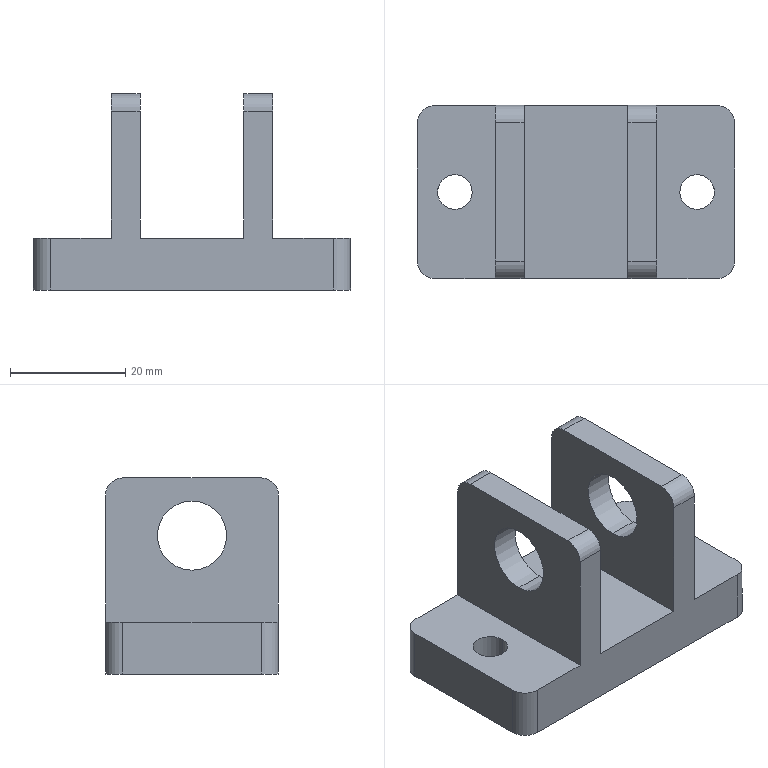Part | STEP file | Hinge seat | 1 solid | 30 faces | box 55 x 30 x 34 mm | volume 20602 mm3 | cylinder 16 | plane 14 | commonest cylinder face diameters 6 x12 12 x4
STEP:
#1=CARTESIAN_POINT('',(-24.,0.,0.));
#2=VERTEX_POINT('',#1);
#3=CARTESIAN_POINT('',(-18.,0.,0.));
#4=VERTEX_POINT('',#3);
#5=CARTESIAN_POINT('',(-21.,0.,0.));
#6=DIRECTION('',(0.,0.,1.));
#7=DIRECTION('',(1.,0.,0.));
#8=AXIS2_PLACEMENT_3D('',#5,#6,#7);
#9=CIRCLE('',#8,3.);
#10=EDGE_CURVE('',#2,#4,#9,.T.);
#11=ORIENTED_EDGE('',*,*,#10,.F.);
#12=CARTESIAN_POINT('',(-24.,0.,9.));
#13=VERTEX_POINT('',#12);
#14=CARTESIAN_POINT('',(-24.,0.,-11.));
#15=DIRECTION('',(0.,0.,1.));
#16=VECTOR('',#15,1000.);
#17=LINE('',#14,#16);
#18=EDGE_CURVE('',#2,#13,#17,.T.);
#19=ORIENTED_EDGE('',*,*,#18,.T.);
#20=CARTESIAN_POINT('',(-18.,0.,9.));
#21=VERTEX_POINT('',#20);
#22=CARTESIAN_POINT('',(-21.,0.,9.));
#23=DIRECTION('',(0.,0.,1.));
#24=DIRECTION('',(1.,0.,0.));
#25=AXIS2_PLACEMENT_3D('',#22,#23,#24);
#26=CIRCLE('',#25,3.);
#27=EDGE_CURVE('',#13,#21,#26,.T.);
#28=ORIENTED_EDGE('',*,*,#27,.T.);
#29=CARTESIAN_POINT('',(-18.,0.,-11.));
#30=DIRECTION('',(0.,0.,1.));
#31=VECTOR('',#30,1000.);
#32=LINE('',#29,#31);
#33=EDGE_CURVE('',#4,#21,#32,.T.);
#34=ORIENTED_EDGE('',*,*,#33,.F.);
#35=EDGE_LOOP('',(#11,#19,#28,#34));
#36=FACE_OUTER_BOUND('',#35,.T.);
#37=CARTESIAN_POINT('',(-21.,0.,-11.));
#38=DIRECTION('',(0.,0.,1.));
#39=DIRECTION('',(1.,0.,0.));
#40=AXIS2_PLACEMENT_3D('',#37,#38,#39);
#41=CYLINDRICAL_SURFACE('',#40,3.);
#42=ADVANCED_FACE('',(#36),#41,.F.);
#43=CARTESIAN_POINT('',(18.,0.,0.));
#44=VERTEX_POINT('',#43);
#45=CARTESIAN_POINT('',(24.,0.,0.));
#46=VERTEX_POINT('',#45);
#47=CARTESIAN_POINT('',(21.,0.,0.));
#48=DIRECTION('',(0.,0.,1.));
#49=DIRECTION('',(1.,0.,0.));
#50=AXIS2_PLACEMENT_3D('',#47,#48,#49);
#51=CIRCLE('',#50,3.);
#52=EDGE_CURVE('',#44,#46,#51,.T.);
#53=ORIENTED_EDGE('',*,*,#52,.F.);
#54=CARTESIAN_POINT('',(18.,0.,9.));
#55=VERTEX_POINT('',#54);
#56=CARTESIAN_POINT('',(18.,0.,-11.));
#57=DIRECTION('',(0.,0.,1.));
#58=VECTOR('',#57,1000.);
#59=LINE('',#56,#58);
#60=EDGE_CURVE('',#44,#55,#59,.T.);
#61=ORIENTED_EDGE('',*,*,#60,.T.);
#62=CARTESIAN_POINT('',(24.,0.,9.));
#63=VERTEX_POINT('',#62);
#64=CARTESIAN_POINT('',(21.,0.,9.));
#65=DIRECTION('',(0.,0.,1.));
#66=DIRECTION('',(1.,0.,0.));
#67=AXIS2_PLACEMENT_3D('',#64,#65,#66);
#68=CIRCLE('',#67,3.);
#69=EDGE_CURVE('',#55,#63,#68,.T.);
#70=ORIENTED_EDGE('',*,*,#69,.T.);
#71=CARTESIAN_POINT('',(24.,0.,-11.));
#72=DIRECTION('',(0.,0.,1.));
#73=VECTOR('',#72,1000.);
#74=LINE('',#71,#73);
#75=EDGE_CURVE('',#46,#63,#74,.T.);
#76=ORIENTED_EDGE('',*,*,#75,.F.);
#77=EDGE_LOOP('',(#53,#61,#70,#76));
#78=FACE_OUTER_BOUND('',#77,.T.);
#79=CARTESIAN_POINT('',(21.,0.,-11.));
#80=DIRECTION('',(0.,0.,1.));
#81=DIRECTION('',(1.,0.,0.));
#82=AXIS2_PLACEMENT_3D('',#79,#80,#81);
#83=CYLINDRICAL_SURFACE('',#82,3.);
#84=ADVANCED_FACE('',(#78),#83,.F.);
#85=CARTESIAN_POINT('',(-9.,0.,18.));
#86=VERTEX_POINT('',#85);
#87=CARTESIAN_POINT('',(-9.,0.,30.));
#88=VERTEX_POINT('',#87);
#89=CARTESIAN_POINT('',(-9.,0.,24.));
#90=DIRECTION('',(-1.,0.,0.));
#91=DIRECTION('',(0.,-1.,0.));
#92=AXIS2_PLACEMENT_3D('',#89,#90,#91);
#93=CIRCLE('',#92,6.);
#94=EDGE_CURVE('',#86,#88,#93,.T.);
#95=ORIENTED_EDGE('',*,*,#94,.F.);
#96=CARTESIAN_POINT('',(-14.,0.,18.));
#97=VERTEX_POINT('',#96);
#98=CARTESIAN_POINT('',(27.5,0.,18.));
#99=DIRECTION('',(-1.,0.,0.));
#100=VECTOR('',#99,1000.);
#101=LINE('',#98,#100);
#102=EDGE_CURVE('',#86,#97,#101,.T.);
#103=ORIENTED_EDGE('',*,*,#102,.T.);
#104=CARTESIAN_POINT('',(-14.,0.,30.));
#105=VERTEX_POINT('',#104);
#106=CARTESIAN_POINT('',(-14.,0.,24.));
#107=DIRECTION('',(-1.,0.,0.));
#108=DIRECTION('',(0.,0.,1.));
#109=AXIS2_PLACEMENT_3D('',#106,#107,#108);
#110=CIRCLE('',#109,6.);
#111=EDGE_CURVE('',#97,#105,#110,.T.);
#112=ORIENTED_EDGE('',*,*,#111,.T.);
#113=CARTESIAN_POINT('',(27.5,0.,30.));
#114=DIRECTION('',(-1.,0.,0.));
#115=VECTOR('',#114,1000.);
#116=LINE('',#113,#115);
#117=EDGE_CURVE('',#88,#105,#116,.T.);
#118=ORIENTED_EDGE('',*,*,#117,.F.);
#119=EDGE_LOOP('',(#95,#103,#112,#118));
#120=FACE_OUTER_BOUND('',#119,.T.);
#121=CARTESIAN_POINT('',(27.5,0.,24.));
#122=DIRECTION('',(-1.,0.,0.));
#123=DIRECTION('',(0.,0.,1.));
#124=AXIS2_PLACEMENT_3D('',#121,#122,#123);
#125=CYLINDRICAL_SURFACE('',#124,6.);
#126=ADVANCED_FACE('',(#120),#125,.F.);
#127=CARTESIAN_POINT('',(14.,0.,18.));
#128=VERTEX_POINT('',#127);
#129=CARTESIAN_POINT('',(14.,0.,30.));
#130=VERTEX_POINT('',#129);
#131=CARTESIAN_POINT('',(14.,0.,24.));
#132=DIRECTION('',(-1.,0.,0.));
#133=DIRECTION('',(0.,-1.,0.));
#134=AXIS2_PLACEMENT_3D('',#131,#132,#133);
#135=CIRCLE('',#134,6.);
#136=EDGE_CURVE('',#128,#130,#135,.T.);
#137=ORIENTED_EDGE('',*,*,#136,.F.);
#138=CARTESIAN_POINT('',(9.,0.,18.));
#139=VERTEX_POINT('',#138);
#140=CARTESIAN_POINT('',(27.5,0.,18.));
#141=DIRECTION('',(-1.,0.,0.));
#142=VECTOR('',#141,1000.);
#143=LINE('',#140,#142);
#144=EDGE_CURVE('',#128,#139,#143,.T.);
#145=ORIENTED_EDGE('',*,*,#144,.T.);
#146=CARTESIAN_POINT('',(9.,0.,30.));
#147=VERTEX_POINT('',#146);
#148=CARTESIAN_POINT('',(9.,0.,24.));
#149=DIRECTION('',(1.,0.,0.));
#150=DIRECTION('',(0.,1.,0.));
#151=AXIS2_PLACEMENT_3D('',#148,#149,#150);
#152=CIRCLE('',#151,6.);
#153=EDGE_CURVE('',#147,#139,#152,.T.);
#154=ORIENTED_EDGE('',*,*,#153,.F.);
#155=CARTESIAN_POINT('',(27.5,0.,30.));
#156=DIRECTION('',(-1.,0.,0.));
#157=VECTOR('',#156,1000.);
#158=LINE('',#155,#157);
#159=EDGE_CURVE('',#130,#147,#158,.T.);
#160=ORIENTED_EDGE('',*,*,#159,.F.);
#161=EDGE_LOOP('',(#137,#145,#154,#160));
#162=FACE_OUTER_BOUND('',#161,.T.);
#163=CARTESIAN_POINT('',(27.5,0.,24.));
#164=DIRECTION('',(-1.,0.,0.));
#165=DIRECTION('',(0.,0.,1.));
#166=AXIS2_PLACEMENT_3D('',#163,#164,#165);
#167=CYLINDRICAL_SURFACE('',#166,6.);
#168=ADVANCED_FACE('',(#162),#167,.F.);
#169=CARTESIAN_POINT('',(-9.,-15.,9.));
#170=VERTEX_POINT('',#169);
#171=CARTESIAN_POINT('',(9.,-15.,9.));
#172=VERTEX_POINT('',#171);
#173=CARTESIAN_POINT('',(-27.5,-15.,9.));
#174=DIRECTION('',(1.,0.,0.));
#175=VECTOR('',#174,1000.);
#176=LINE('',#173,#175);
#177=EDGE_CURVE('',#170,#172,#176,.T.);
#178=ORIENTED_EDGE('',*,*,#177,.T.);
#179=CARTESIAN_POINT('',(9.,15.,9.));
#180=VERTEX_POINT('',#179);
#181=CARTESIAN_POINT('',(9.,15.,9.));
#182=DIRECTION('',(0.,-1.,0.));
#183=VECTOR('',#182,1000.);
#184=LINE('',#181,#183);
#185=EDGE_CURVE('',#180,#172,#184,.T.);
#186=ORIENTED_EDGE('',*,*,#185,.F.);
#187=CARTESIAN_POINT('',(-9.,15.,9.));
#188=VERTEX_POINT('',#187);
#189=CARTESIAN_POINT('',(-27.5,15.,9.));
#190=DIRECTION('',(-1.,0.,0.));
#191=VECTOR('',#190,1000.);
#192=LINE('',#189,#191);
#193=EDGE_CURVE('',#180,#188,#192,.T.);
#194=ORIENTED_EDGE('',*,*,#193,.T.);
#195=CARTESIAN_POINT('',(-9.,15.,9.));
#196=DIRECTION('',(0.,1.,0.));
#197=VECTOR('',#196,1000.);
#198=LINE('',#195,#197);
#199=EDGE_CURVE('',#170,#188,#198,.T.);
#200=ORIENTED_EDGE('',*,*,#199,.F.);
#201=EDGE_LOOP('',(#178,#186,#194,#200));
#202=FACE_OUTER_BOUND('',#201,.T.);
#203=CARTESIAN_POINT('',(0.,0.,9.));
#204=DIRECTION('',(0.,0.,1.));
#205=DIRECTION('',(1.,0.,0.));
#206=AXIS2_PLACEMENT_3D('',#203,#204,#205);
#207=PLANE('',#206);
#208=ADVANCED_FACE('',(#202),#207,.T.);
#209=CARTESIAN_POINT('',(21.,0.,9.));
#210=DIRECTION('',(0.,0.,1.));
#211=DIRECTION('',(1.,0.,0.));
#212=AXIS2_PLACEMENT_3D('',#209,#210,#211);
#213=CIRCLE('',#212,3.);
#214=EDGE_CURVE('',#63,#55,#213,.T.);
#215=ORIENTED_EDGE('',*,*,#214,.F.);
#216=ORIENTED_EDGE('',*,*,#69,.F.);
#217=EDGE_LOOP('',(#215,#216));
#218=FACE_BOUND('',#217,.T.);
#219=CARTESIAN_POINT('',(24.5,15.,9.));
#220=VERTEX_POINT('',#219);
#221=CARTESIAN_POINT('',(14.,15.,9.));
#222=VERTEX_POINT('',#221);
#223=CARTESIAN_POINT('',(-27.5,15.,9.));
#224=DIRECTION('',(-1.,0.,0.));
#225=VECTOR('',#224,1000.);
#226=LINE('',#223,#225);
#227=EDGE_CURVE('',#220,#222,#226,.T.);
#228=ORIENTED_EDGE('',*,*,#227,.T.);
#229=CARTESIAN_POINT('',(14.,-15.,9.));
#230=VERTEX_POINT('',#229);
#231=CARTESIAN_POINT('',(14.,15.,9.));
#232=DIRECTION('',(0.,1.,0.));
#233=VECTOR('',#232,1000.);
#234=LINE('',#231,#233);
#235=EDGE_CURVE('',#230,#222,#234,.T.);
#236=ORIENTED_EDGE('',*,*,#235,.F.);
#237=CARTESIAN_POINT('',(24.5,-15.,9.));
#238=VERTEX_POINT('',#237);
#239=CARTESIAN_POINT('',(-27.5,-15.,9.));
#240=DIRECTION('',(1.,0.,0.));
#241=VECTOR('',#240,1000.);
#242=LINE('',#239,#241);
#243=EDGE_CURVE('',#230,#238,#242,.T.);
#244=ORIENTED_EDGE('',*,*,#243,.T.);
#245=CARTESIAN_POINT('',(27.5,-12.,9.));
#246=VERTEX_POINT('',#245);
#247=CARTESIAN_POINT('',(24.5,-12.,9.));
#248=DIRECTION('',(0.,0.,1.));
#249=DIRECTION('',(1.,0.,0.));
#250=AXIS2_PLACEMENT_3D('',#247,#248,#249);
#251=CIRCLE('',#250,3.);
#252=EDGE_CURVE('',#238,#246,#251,.T.);
#253=ORIENTED_EDGE('',*,*,#252,.T.);
#254=CARTESIAN_POINT('',(27.5,12.,9.));
#255=VERTEX_POINT('',#254);
#256=CARTESIAN_POINT('',(27.5,15.,9.));
#257=DIRECTION('',(0.,1.,0.));
#258=VECTOR('',#257,1000.);
#259=LINE('',#256,#258);
#260=EDGE_CURVE('',#246,#255,#259,.T.);
#261=ORIENTED_EDGE('',*,*,#260,.T.);
#262=CARTESIAN_POINT('',(24.5,12.,9.));
#263=DIRECTION('',(0.,0.,1.));
#264=DIRECTION('',(1.,0.,0.));
#265=AXIS2_PLACEMENT_3D('',#262,#263,#264);
#266=CIRCLE('',#265,3.);
#267=EDGE_CURVE('',#255,#220,#266,.T.);
#268=ORIENTED_EDGE('',*,*,#267,.T.);
#269=EDGE_LOOP('',(#228,#236,#244,#253,#261,#268));
#270=FACE_OUTER_BOUND('',#269,.T.);
#271=CARTESIAN_POINT('',(0.,0.,9.));
#272=DIRECTION('',(0.,0.,1.));
#273=DIRECTION('',(1.,0.,0.));
#274=AXIS2_PLACEMENT_3D('',#271,#272,#273);
#275=PLANE('',#274);
#276=ADVANCED_FACE('',(#218,#270),#275,.T.);
#277=CARTESIAN_POINT('',(-21.,0.,9.));
#278=DIRECTION('',(0.,0.,1.));
#279=DIRECTION('',(1.,0.,0.));
#280=AXIS2_PLACEMENT_3D('',#277,#278,#279);
#281=CIRCLE('',#280,3.);
#282=EDGE_CURVE('',#21,#13,#281,.T.);
#283=ORIENTED_EDGE('',*,*,#282,.F.);
#284=ORIENTED_EDGE('',*,*,#27,.F.);
#285=EDGE_LOOP('',(#283,#284));
#286=FACE_BOUND('',#285,.T.);
#287=CARTESIAN_POINT('',(-14.,15.,9.));
#288=VERTEX_POINT('',#287);
#289=CARTESIAN_POINT('',(-14.,-15.,9.));
#290=VERTEX_POINT('',#289);
#291=CARTESIAN_POINT('',(-14.,15.,9.));
#292=DIRECTION('',(0.,-1.,0.));
#293=VECTOR('',#292,1000.);
#294=LINE('',#291,#293);
#295=EDGE_CURVE('',#288,#290,#294,.T.);
#296=ORIENTED_EDGE('',*,*,#295,.F.);
#297=CARTESIAN_POINT('',(-24.5,15.,9.));
#298=VERTEX_POINT('',#297);
#299=CARTESIAN_POINT('',(-27.5,15.,9.));
#300=DIRECTION('',(-1.,0.,0.));
#301=VECTOR('',#300,1000.);
#302=LINE('',#299,#301);
#303=EDGE_CURVE('',#288,#298,#302,.T.);
#304=ORIENTED_EDGE('',*,*,#303,.T.);
#305=CARTESIAN_POINT('',(-27.5,12.,9.));
#306=VERTEX_POINT('',#305);
#307=CARTESIAN_POINT('',(-24.5,12.,9.));
#308=DIRECTION('',(0.,0.,1.));
#309=DIRECTION('',(1.,0.,0.));
#310=AXIS2_PLACEMENT_3D('',#307,#308,#309);
#311=CIRCLE('',#310,3.);
#312=EDGE_CURVE('',#298,#306,#311,.T.);
#313=ORIENTED_EDGE('',*,*,#312,.T.);
#314=CARTESIAN_POINT('',(-27.5,-12.,9.));
#315=VERTEX_POINT('',#314);
#316=CARTESIAN_POINT('',(-27.5,15.,9.));
#317=DIRECTION('',(0.,-1.,0.));
#318=VECTOR('',#317,1000.);
#319=LINE('',#316,#318);
#320=EDGE_CURVE('',#306,#315,#319,.T.);
#321=ORIENTED_EDGE('',*,*,#320,.T.);
#322=CARTESIAN_POINT('',(-24.5,-15.,9.));
#323=VERTEX_POINT('',#322);
#324=CARTESIAN_POINT('',(-24.5,-12.,9.));
#325=DIRECTION('',(0.,0.,1.));
#326=DIRECTION('',(1.,0.,0.));
#327=AXIS2_PLACEMENT_3D('',#324,#325,#326);
#328=CIRCLE('',#327,3.);
#329=EDGE_CURVE('',#315,#323,#328,.T.);
#330=ORIENTED_EDGE('',*,*,#329,.T.);
#331=CARTESIAN_POINT('',(-27.5,-15.,9.));
#332=DIRECTION('',(1.,0.,0.));
#333=VECTOR('',#332,1000.);
#334=LINE('',#331,#333);
#335=EDGE_CURVE('',#323,#290,#334,.T.);
#336=ORIENTED_EDGE('',*,*,#335,.T.);
#337=EDGE_LOOP('',(#296,#304,#313,#321,#330,#336));
#338=FACE_OUTER_BOUND('',#337,.T.);
#339=CARTESIAN_POINT('',(0.,0.,9.));
#340=DIRECTION('',(0.,0.,1.));
#341=DIRECTION('',(1.,0.,0.));
#342=AXIS2_PLACEMENT_3D('',#339,#340,#341);
#343=PLANE('',#342);
#344=ADVANCED_FACE('',(#286,#338),#343,.T.);
#345=CARTESIAN_POINT('',(27.5,-12.,0.));
#346=VERTEX_POINT('',#345);
#347=CARTESIAN_POINT('',(27.5,12.,0.));
#348=VERTEX_POINT('',#347);
#349=CARTESIAN_POINT('',(27.5,15.,0.));
#350=DIRECTION('',(0.,1.,0.));
#351=VECTOR('',#350,1000.);
#352=LINE('',#349,#351);
#353=EDGE_CURVE('',#346,#348,#352,.T.);
#354=ORIENTED_EDGE('',*,*,#353,.T.);
#355=CARTESIAN_POINT('',(27.5,12.,9.));
#356=DIRECTION('',(0.,0.,1.));
#357=VECTOR('',#356,1000.);
#358=LINE('',#355,#357);
#359=EDGE_CURVE('',#348,#255,#358,.T.);
#360=ORIENTED_EDGE('',*,*,#359,.T.);
#361=ORIENTED_EDGE('',*,*,#260,.F.);
#362=CARTESIAN_POINT('',(27.5,-12.,9.));
#363=DIRECTION('',(0.,0.,-1.));
#364=VECTOR('',#363,1000.);
#365=LINE('',#362,#364);
#366=EDGE_CURVE('',#246,#346,#365,.T.);
#367=ORIENTED_EDGE('',*,*,#366,.T.);
#368=EDGE_LOOP('',(#354,#360,#361,#367));
#369=FACE_OUTER_BOUND('',#368,.T.);
#370=CARTESIAN_POINT('',(27.5,15.,9.));
#371=DIRECTION('',(-1.,0.,0.));
#372=DIRECTION('',(0.,-1.,0.));
#373=AXIS2_PLACEMENT_3D('',#370,#371,#372);
#374=PLANE('',#373);
#375=ADVANCED_FACE('',(#369),#374,.F.);
#376=CARTESIAN_POINT('',(9.,15.,31.));
#377=VERTEX_POINT('',#376);
#378=CARTESIAN_POINT('',(9.,15.,34.));
#379=DIRECTION('',(0.,0.,-1.));
#380=VECTOR('',#379,1000.);
#381=LINE('',#378,#380);
#382=EDGE_CURVE('',#377,#180,#381,.T.);
#383=ORIENTED_EDGE('',*,*,#382,.F.);
#384=CARTESIAN_POINT('',(14.,15.,31.));
#385=VERTEX_POINT('',#384);
#386=CARTESIAN_POINT('',(14.,15.,31.));
#387=DIRECTION('',(1.,0.,0.));
#388=VECTOR('',#387,1000.);
#389=LINE('',#386,#388);
#390=EDGE_CURVE('',#377,#385,#389,.T.);
#391=ORIENTED_EDGE('',*,*,#390,.T.);
#392=CARTESIAN_POINT('',(14.,15.,34.));
#393=DIRECTION('',(0.,0.,-1.));
#394=VECTOR('',#393,1000.);
#395=LINE('',#392,#394);
#396=EDGE_CURVE('',#385,#222,#395,.T.);
#397=ORIENTED_EDGE('',*,*,#396,.T.);
#398=ORIENTED_EDGE('',*,*,#227,.F.);
#399=CARTESIAN_POINT('',(24.5,15.,0.));
#400=VERTEX_POINT('',#399);
#401=CARTESIAN_POINT('',(24.5,15.,9.));
#402=DIRECTION('',(0.,0.,-1.));
#403=VECTOR('',#402,1000.);
#404=LINE('',#401,#403);
#405=EDGE_CURVE('',#220,#400,#404,.T.);
#406=ORIENTED_EDGE('',*,*,#405,.T.);
#407=CARTESIAN_POINT('',(-24.5,15.,0.));
#408=VERTEX_POINT('',#407);
#409=CARTESIAN_POINT('',(-27.5,15.,0.));
#410=DIRECTION('',(-1.,0.,0.));
#411=VECTOR('',#410,1000.);
#412=LINE('',#409,#411);
#413=EDGE_CURVE('',#400,#408,#412,.T.);
#414=ORIENTED_EDGE('',*,*,#413,.T.);
#415=CARTESIAN_POINT('',(-24.5,15.,9.));
#416=DIRECTION('',(0.,0.,1.));
#417=VECTOR('',#416,1000.);
#418=LINE('',#415,#417);
#419=EDGE_CURVE('',#408,#298,#418,.T.);
#420=ORIENTED_EDGE('',*,*,#419,.T.);
#421=ORIENTED_EDGE('',*,*,#303,.F.);
#422=CARTESIAN_POINT('',(-14.,15.,31.));
#423=VERTEX_POINT('',#422);
#424=CARTESIAN_POINT('',(-14.,15.,34.));
#425=DIRECTION('',(0.,0.,-1.));
#426=VECTOR('',#425,1000.);
#427=LINE('',#424,#426);
#428=EDGE_CURVE('',#423,#288,#427,.T.);
#429=ORIENTED_EDGE('',*,*,#428,.F.);
#430=CARTESIAN_POINT('',(-9.,15.,31.));
#431=VERTEX_POINT('',#430);
#432=CARTESIAN_POINT('',(-9.,15.,31.));
#433=DIRECTION('',(1.,0.,0.));
#434=VECTOR('',#433,1000.);
#435=LINE('',#432,#434);
#436=EDGE_CURVE('',#423,#431,#435,.T.);
#437=ORIENTED_EDGE('',*,*,#436,.T.);
#438=CARTESIAN_POINT('',(-9.,15.,34.));
#439=DIRECTION('',(0.,0.,-1.));
#440=VECTOR('',#439,1000.);
#441=LINE('',#438,#440);
#442=EDGE_CURVE('',#431,#188,#441,.T.);
#443=ORIENTED_EDGE('',*,*,#442,.T.);
#444=ORIENTED_EDGE('',*,*,#193,.F.);
#445=EDGE_LOOP('',(#383,#391,#397,#398,#406,#414,#420,#421,#429,#437,#443,#444));
#446=FACE_OUTER_BOUND('',#445,.T.);
#447=CARTESIAN_POINT('',(-27.5,15.,9.));
#448=DIRECTION('',(0.,-1.,0.));
#449=DIRECTION('',(0.,0.,-1.));
#450=AXIS2_PLACEMENT_3D('',#447,#448,#449);
#451=PLANE('',#450);
#452=ADVANCED_FACE('',(#446),#451,.F.);
#453=ORIENTED_EDGE('',*,*,#320,.F.);
#454=CARTESIAN_POINT('',(-27.5,12.,0.));
#455=VERTEX_POINT('',#454);
#456=CARTESIAN_POINT('',(-27.5,12.,9.));
#457=DIRECTION('',(0.,0.,-1.));
#458=VECTOR('',#457,1000.);
#459=LINE('',#456,#458);
#460=EDGE_CURVE('',#306,#455,#459,.T.);
#461=ORIENTED_EDGE('',*,*,#460,.T.);
#462=CARTESIAN_POINT('',(-27.5,-12.,0.));
#463=VERTEX_POINT('',#462);
#464=CARTESIAN_POINT('',(-27.5,15.,0.));
#465=DIRECTION('',(0.,-1.,0.));
#466=VECTOR('',#465,1000.);
#467=LINE('',#464,#466);
#468=EDGE_CURVE('',#455,#463,#467,.T.);
#469=ORIENTED_EDGE('',*,*,#468,.T.);
#470=CARTESIAN_POINT('',(-27.5,-12.,9.));
#471=DIRECTION('',(0.,0.,1.));
#472=VECTOR('',#471,1000.);
#473=LINE('',#470,#472);
#474=EDGE_CURVE('',#463,#315,#473,.T.);
#475=ORIENTED_EDGE('',*,*,#474,.T.);
#476=EDGE_LOOP('',(#453,#461,#469,#475));
#477=FACE_OUTER_BOUND('',#476,.T.);
#478=CARTESIAN_POINT('',(-27.5,15.,9.));
#479=DIRECTION('',(1.,0.,0.));
#480=DIRECTION('',(0.,1.,0.));
#481=AXIS2_PLACEMENT_3D('',#478,#479,#480);
#482=PLANE('',#481);
#483=ADVANCED_FACE('',(#477),#482,.F.);
#484=CARTESIAN_POINT('',(14.,-15.,31.));
#485=VERTEX_POINT('',#484);
#486=CARTESIAN_POINT('',(14.,-15.,34.));
#487=DIRECTION('',(0.,0.,-1.));
#488=VECTOR('',#487,1000.);
#489=LINE('',#486,#488);
#490=EDGE_CURVE('',#485,#230,#489,.T.);
#491=ORIENTED_EDGE('',*,*,#490,.F.);
#492=CARTESIAN_POINT('',(9.,-15.,31.));
#493=VERTEX_POINT('',#492);
#494=CARTESIAN_POINT('',(9.,-15.,31.));
#495=DIRECTION('',(-1.,0.,0.));
#496=VECTOR('',#495,1000.);
#497=LINE('',#494,#496);
#498=EDGE_CURVE('',#485,#493,#497,.T.);
#499=ORIENTED_EDGE('',*,*,#498,.T.);
#500=CARTESIAN_POINT('',(9.,-15.,34.));
#501=DIRECTION('',(0.,0.,-1.));
#502=VECTOR('',#501,1000.);
#503=LINE('',#500,#502);
#504=EDGE_CURVE('',#493,#172,#503,.T.);
#505=ORIENTED_EDGE('',*,*,#504,.T.);
#506=ORIENTED_EDGE('',*,*,#177,.F.);
#507=CARTESIAN_POINT('',(-9.,-15.,31.));
#508=VERTEX_POINT('',#507);
#509=CARTESIAN_POINT('',(-9.,-15.,34.));
#510=DIRECTION('',(0.,0.,-1.));
#511=VECTOR('',#510,1000.);
#512=LINE('',#509,#511);
#513=EDGE_CURVE('',#508,#170,#512,.T.);
#514=ORIENTED_EDGE('',*,*,#513,.F.);
#515=CARTESIAN_POINT('',(-14.,-15.,31.));
#516=VERTEX_POINT('',#515);
#517=CARTESIAN_POINT('',(-14.,-15.,31.));
#518=DIRECTION('',(-1.,0.,0.));
#519=VECTOR('',#518,1000.);
#520=LINE('',#517,#519);
#521=EDGE_CURVE('',#508,#516,#520,.T.);
#522=ORIENTED_EDGE('',*,*,#521,.T.);
#523=CARTESIAN_POINT('',(-14.,-15.,34.));
#524=DIRECTION('',(0.,0.,-1.));
#525=VECTOR('',#524,1000.);
#526=LINE('',#523,#525);
#527=EDGE_CURVE('',#516,#290,#526,.T.);
#528=ORIENTED_EDGE('',*,*,#527,.T.);
#529=ORIENTED_EDGE('',*,*,#335,.F.);
#530=CARTESIAN_POINT('',(-24.5,-15.,0.));
#531=VERTEX_POINT('',#530);
#532=CARTESIAN_POINT('',(-24.5,-15.,9.));
#533=DIRECTION('',(0.,0.,-1.));
#534=VECTOR('',#533,1000.);
#535=LINE('',#532,#534);
#536=EDGE_CURVE('',#323,#531,#535,.T.);
#537=ORIENTED_EDGE('',*,*,#536,.T.);
#538=CARTESIAN_POINT('',(24.5,-15.,0.));
#539=VERTEX_POINT('',#538);
#540=CARTESIAN_POINT('',(-27.5,-15.,0.));
#541=DIRECTION('',(1.,0.,0.));
#542=VECTOR('',#541,1000.);
#543=LINE('',#540,#542);
#544=EDGE_CURVE('',#531,#539,#543,.T.);
#545=ORIENTED_EDGE('',*,*,#544,.T.);
#546=CARTESIAN_POINT('',(24.5,-15.,9.));
#547=DIRECTION('',(0.,0.,1.));
#548=VECTOR('',#547,1000.);
#549=LINE('',#546,#548);
#550=EDGE_CURVE('',#539,#238,#549,.T.);
#551=ORIENTED_EDGE('',*,*,#550,.T.);
#552=ORIENTED_EDGE('',*,*,#243,.F.);
#553=EDGE_LOOP('',(#491,#499,#505,#506,#514,#522,#528,#529,#537,#545,#551,#552));
#554=FACE_OUTER_BOUND('',#553,.T.);
#555=CARTESIAN_POINT('',(-27.5,-15.,9.));
#556=DIRECTION('',(0.,1.,0.));
#557=DIRECTION('',(0.,0.,1.));
#558=AXIS2_PLACEMENT_3D('',#555,#556,#557);
#559=PLANE('',#558);
#560=ADVANCED_FACE('',(#554),#559,.F.);
#561=CARTESIAN_POINT('',(-21.,0.,0.));
#562=DIRECTION('',(0.,0.,1.));
#563=DIRECTION('',(1.,0.,0.));
#564=AXIS2_PLACEMENT_3D('',#561,#562,#563);
#565=CIRCLE('',#564,3.);
#566=EDGE_CURVE('',#4,#2,#565,.T.);
#567=ORIENTED_EDGE('',*,*,#566,.T.);
#568=ORIENTED_EDGE('',*,*,#10,.T.);
#569=EDGE_LOOP('',(#567,#568));
#570=FACE_BOUND('',#569,.T.);
#571=CARTESIAN_POINT('',(21.,0.,0.));
#572=DIRECTION('',(0.,0.,1.));
#573=DIRECTION('',(1.,0.,0.));
#574=AXIS2_PLACEMENT_3D('',#571,#572,#573);
#575=CIRCLE('',#574,3.);
#576=EDGE_CURVE('',#46,#44,#575,.T.);
#577=ORIENTED_EDGE('',*,*,#576,.T.);
#578=ORIENTED_EDGE('',*,*,#52,.T.);
#579=EDGE_LOOP('',(#577,#578));
#580=FACE_BOUND('',#579,.T.);
#581=ORIENTED_EDGE('',*,*,#413,.F.);
#582=CARTESIAN_POINT('',(24.5,12.,0.));
#583=DIRECTION('',(0.,0.,-1.));
#584=DIRECTION('',(1.,0.,0.));
#585=AXIS2_PLACEMENT_3D('',#582,#583,#584);
#586=CIRCLE('',#585,3.);
#587=EDGE_CURVE('',#400,#348,#586,.T.);
#588=ORIENTED_EDGE('',*,*,#587,.T.);
#589=ORIENTED_EDGE('',*,*,#353,.F.);
#590=CARTESIAN_POINT('',(24.5,-12.,0.));
#591=DIRECTION('',(0.,0.,-1.));
#592=DIRECTION('',(1.,0.,0.));
#593=AXIS2_PLACEMENT_3D('',#590,#591,#592);
#594=CIRCLE('',#593,3.);
#595=EDGE_CURVE('',#346,#539,#594,.T.);
#596=ORIENTED_EDGE('',*,*,#595,.T.);
#597=ORIENTED_EDGE('',*,*,#544,.F.);
#598=CARTESIAN_POINT('',(-24.5,-12.,0.));
#599=DIRECTION('',(0.,0.,-1.));
#600=DIRECTION('',(1.,0.,0.));
#601=AXIS2_PLACEMENT_3D('',#598,#599,#600);
#602=CIRCLE('',#601,3.);
#603=EDGE_CURVE('',#531,#463,#602,.T.);
#604=ORIENTED_EDGE('',*,*,#603,.T.);
#605=ORIENTED_EDGE('',*,*,#468,.F.);
#606=CARTESIAN_POINT('',(-24.5,12.,0.));
#607=DIRECTION('',(0.,0.,-1.));
#608=DIRECTION('',(1.,0.,0.));
#609=AXIS2_PLACEMENT_3D('',#606,#607,#608);
#610=CIRCLE('',#609,3.);
#611=EDGE_CURVE('',#455,#408,#610,.T.);
#612=ORIENTED_EDGE('',*,*,#611,.T.);
#613=EDGE_LOOP('',(#581,#588,#589,#596,#597,#604,#605,#612));
#614=FACE_OUTER_BOUND('',#613,.T.);
#615=CARTESIAN_POINT('',(0.,0.,0.));
#616=DIRECTION('',(0.,0.,1.));
#617=DIRECTION('',(1.,0.,0.));
#618=AXIS2_PLACEMENT_3D('',#615,#616,#617);
#619=PLANE('',#618);
#620=ADVANCED_FACE('',(#570,#580,#614),#619,.F.);
#621=ORIENTED_EDGE('',*,*,#267,.F.);
#622=ORIENTED_EDGE('',*,*,#359,.F.);
#623=ORIENTED_EDGE('',*,*,#587,.F.);
#624=ORIENTED_EDGE('',*,*,#405,.F.);
#625=EDGE_LOOP('',(#621,#622,#623,#624));
#626=FACE_OUTER_BOUND('',#625,.T.);
#627=CARTESIAN_POINT('',(24.5,12.,9.));
#628=DIRECTION('',(0.,0.,-1.));
#629=DIRECTION('',(-1.,0.,0.));
#630=AXIS2_PLACEMENT_3D('',#627,#628,#629);
#631=CYLINDRICAL_SURFACE('',#630,3.);
#632=ADVANCED_FACE('',(#626),#631,.T.);
#633=ORIENTED_EDGE('',*,*,#252,.F.);
#634=ORIENTED_EDGE('',*,*,#550,.F.);
#635=ORIENTED_EDGE('',*,*,#595,.F.);
#636=ORIENTED_EDGE('',*,*,#366,.F.);
#637=EDGE_LOOP('',(#633,#634,#635,#636));
#638=FACE_OUTER_BOUND('',#637,.T.);
#639=CARTESIAN_POINT('',(24.5,-12.,9.));
#640=DIRECTION('',(0.,0.,-1.));
#641=DIRECTION('',(-1.,0.,0.));
#642=AXIS2_PLACEMENT_3D('',#639,#640,#641);
#643=CYLINDRICAL_SURFACE('',#642,3.);
#644=ADVANCED_FACE('',(#638),#643,.T.);
#645=ORIENTED_EDGE('',*,*,#312,.F.);
#646=ORIENTED_EDGE('',*,*,#419,.F.);
#647=ORIENTED_EDGE('',*,*,#611,.F.);
#648=ORIENTED_EDGE('',*,*,#460,.F.);
#649=EDGE_LOOP('',(#645,#646,#647,#648));
#650=FACE_OUTER_BOUND('',#649,.T.);
#651=CARTESIAN_POINT('',(-24.5,12.,9.));
#652=DIRECTION('',(0.,0.,-1.));
#653=DIRECTION('',(-1.,0.,0.));
#654=AXIS2_PLACEMENT_3D('',#651,#652,#653);
#655=CYLINDRICAL_SURFACE('',#654,3.);
#656=ADVANCED_FACE('',(#650),#655,.T.);
#657=ORIENTED_EDGE('',*,*,#329,.F.);
#658=ORIENTED_EDGE('',*,*,#474,.F.);
#659=ORIENTED_EDGE('',*,*,#603,.F.);
#660=ORIENTED_EDGE('',*,*,#536,.F.);
#661=EDGE_LOOP('',(#657,#658,#659,#660));
#662=FACE_OUTER_BOUND('',#661,.T.);
#663=CARTESIAN_POINT('',(-24.5,-12.,9.));
#664=DIRECTION('',(0.,0.,-1.));
#665=DIRECTION('',(-1.,0.,0.));
#666=AXIS2_PLACEMENT_3D('',#663,#664,#665);
#667=CYLINDRICAL_SURFACE('',#666,3.);
#668=ADVANCED_FACE('',(#662),#667,.T.);
#669=CARTESIAN_POINT('',(-14.,0.,24.));
#670=DIRECTION('',(-1.,0.,0.));
#671=DIRECTION('',(0.,0.,1.));
#672=AXIS2_PLACEMENT_3D('',#669,#670,#671);
#673=CIRCLE('',#672,6.);
#674=EDGE_CURVE('',#105,#97,#673,.T.);
#675=ORIENTED_EDGE('',*,*,#674,.F.);
#676=ORIENTED_EDGE('',*,*,#111,.F.);
#677=EDGE_LOOP('',(#675,#676));
#678=FACE_BOUND('',#677,.T.);
#679=ORIENTED_EDGE('',*,*,#527,.F.);
#680=CARTESIAN_POINT('',(-14.,-12.,34.));
#681=VERTEX_POINT('',#680);
#682=CARTESIAN_POINT('',(-14.,-12.,31.));
#683=DIRECTION('',(-1.,0.,0.));
#684=DIRECTION('',(0.,1.,0.));
#685=AXIS2_PLACEMENT_3D('',#682,#683,#684);
#686=CIRCLE('',#685,3.);
#687=EDGE_CURVE('',#516,#681,#686,.T.);
#688=ORIENTED_EDGE('',*,*,#687,.T.);
#689=CARTESIAN_POINT('',(-14.,12.,34.));
#690=VERTEX_POINT('',#689);
#691=CARTESIAN_POINT('',(-14.,15.,34.));
#692=DIRECTION('',(0.,-1.,0.));
#693=VECTOR('',#692,1000.);
#694=LINE('',#691,#693);
#695=EDGE_CURVE('',#690,#681,#694,.T.);
#696=ORIENTED_EDGE('',*,*,#695,.F.);
#697=CARTESIAN_POINT('',(-14.,12.,31.));
#698=DIRECTION('',(-1.,0.,0.));
#699=DIRECTION('',(0.,1.,0.));
#700=AXIS2_PLACEMENT_3D('',#697,#698,#699);
#701=CIRCLE('',#700,3.);
#702=EDGE_CURVE('',#690,#423,#701,.T.);
#703=ORIENTED_EDGE('',*,*,#702,.T.);
#704=ORIENTED_EDGE('',*,*,#428,.T.);
#705=ORIENTED_EDGE('',*,*,#295,.T.);
#706=EDGE_LOOP('',(#679,#688,#696,#703,#704,#705));
#707=FACE_OUTER_BOUND('',#706,.T.);
#708=CARTESIAN_POINT('',(-14.,15.,34.));
#709=DIRECTION('',(1.,0.,0.));
#710=DIRECTION('',(0.,1.,0.));
#711=AXIS2_PLACEMENT_3D('',#708,#709,#710);
#712=PLANE('',#711);
#713=ADVANCED_FACE('',(#678,#707),#712,.F.);
#714=CARTESIAN_POINT('',(-9.,0.,24.));
#715=DIRECTION('',(-1.,0.,0.));
#716=DIRECTION('',(0.,-1.,0.));
#717=AXIS2_PLACEMENT_3D('',#714,#715,#716);
#718=CIRCLE('',#717,6.);
#719=EDGE_CURVE('',#88,#86,#718,.T.);
#720=ORIENTED_EDGE('',*,*,#719,.T.);
#721=ORIENTED_EDGE('',*,*,#94,.T.);
#722=EDGE_LOOP('',(#720,#721));
#723=FACE_BOUND('',#722,.T.);
#724=CARTESIAN_POINT('',(-9.,-12.,34.));
#725=VERTEX_POINT('',#724);
#726=CARTESIAN_POINT('',(-9.,12.,34.));
#727=VERTEX_POINT('',#726);
#728=CARTESIAN_POINT('',(-9.,15.,34.));
#729=DIRECTION('',(0.,1.,0.));
#730=VECTOR('',#729,1000.);
#731=LINE('',#728,#730);
#732=EDGE_CURVE('',#725,#727,#731,.T.);
#733=ORIENTED_EDGE('',*,*,#732,.F.);
#734=CARTESIAN_POINT('',(-9.,-12.,31.));
#735=DIRECTION('',(1.,0.,0.));
#736=DIRECTION('',(0.,-1.,0.));
#737=AXIS2_PLACEMENT_3D('',#734,#735,#736);
#738=CIRCLE('',#737,3.);
#739=EDGE_CURVE('',#725,#508,#738,.T.);
#740=ORIENTED_EDGE('',*,*,#739,.T.);
#741=ORIENTED_EDGE('',*,*,#513,.T.);
#742=ORIENTED_EDGE('',*,*,#199,.T.);
#743=ORIENTED_EDGE('',*,*,#442,.F.);
#744=CARTESIAN_POINT('',(-9.,12.,31.));
#745=DIRECTION('',(1.,0.,0.));
#746=DIRECTION('',(0.,-1.,0.));
#747=AXIS2_PLACEMENT_3D('',#744,#745,#746);
#748=CIRCLE('',#747,3.);
#749=EDGE_CURVE('',#431,#727,#748,.T.);
#750=ORIENTED_EDGE('',*,*,#749,.T.);
#751=EDGE_LOOP('',(#733,#740,#741,#742,#743,#750));
#752=FACE_OUTER_BOUND('',#751,.T.);
#753=CARTESIAN_POINT('',(-9.,15.,34.));
#754=DIRECTION('',(-1.,0.,0.));
#755=DIRECTION('',(0.,-1.,0.));
#756=AXIS2_PLACEMENT_3D('',#753,#754,#755);
#757=PLANE('',#756);
#758=ADVANCED_FACE('',(#723,#752),#757,.F.);
#759=ORIENTED_EDGE('',*,*,#695,.T.);
#760=CARTESIAN_POINT('',(-9.,-12.,34.));
#761=DIRECTION('',(1.,0.,0.));
#762=VECTOR('',#761,1000.);
#763=LINE('',#760,#762);
#764=EDGE_CURVE('',#681,#725,#763,.T.);
#765=ORIENTED_EDGE('',*,*,#764,.T.);
#766=ORIENTED_EDGE('',*,*,#732,.T.);
#767=CARTESIAN_POINT('',(-14.,12.,34.));
#768=DIRECTION('',(-1.,0.,0.));
#769=VECTOR('',#768,1000.);
#770=LINE('',#767,#769);
#771=EDGE_CURVE('',#727,#690,#770,.T.);
#772=ORIENTED_EDGE('',*,*,#771,.T.);
#773=EDGE_LOOP('',(#759,#765,#766,#772));
#774=FACE_OUTER_BOUND('',#773,.T.);
#775=CARTESIAN_POINT('',(0.,0.,34.));
#776=DIRECTION('',(0.,0.,1.));
#777=DIRECTION('',(1.,0.,0.));
#778=AXIS2_PLACEMENT_3D('',#775,#776,#777);
#779=PLANE('',#778);
#780=ADVANCED_FACE('',(#774),#779,.T.);
#781=ORIENTED_EDGE('',*,*,#153,.T.);
#782=CARTESIAN_POINT('',(9.,0.,24.));
#783=DIRECTION('',(1.,0.,0.));
#784=DIRECTION('',(0.,1.,0.));
#785=AXIS2_PLACEMENT_3D('',#782,#783,#784);
#786=CIRCLE('',#785,6.);
#787=EDGE_CURVE('',#139,#147,#786,.T.);
#788=ORIENTED_EDGE('',*,*,#787,.T.);
#789=EDGE_LOOP('',(#781,#788));
#790=FACE_BOUND('',#789,.T.);
#791=ORIENTED_EDGE('',*,*,#504,.F.);
#792=CARTESIAN_POINT('',(9.,-12.,34.));
#793=VERTEX_POINT('',#792);
#794=CARTESIAN_POINT('',(9.,-12.,31.));
#795=DIRECTION('',(-1.,0.,0.));
#796=DIRECTION('',(0.,1.,0.));
#797=AXIS2_PLACEMENT_3D('',#794,#795,#796);
#798=CIRCLE('',#797,3.);
#799=EDGE_CURVE('',#493,#793,#798,.T.);
#800=ORIENTED_EDGE('',*,*,#799,.T.);
#801=CARTESIAN_POINT('',(9.,12.,34.));
#802=VERTEX_POINT('',#801);
#803=CARTESIAN_POINT('',(9.,15.,34.));
#804=DIRECTION('',(0.,-1.,0.));
#805=VECTOR('',#804,1000.);
#806=LINE('',#803,#805);
#807=EDGE_CURVE('',#802,#793,#806,.T.);
#808=ORIENTED_EDGE('',*,*,#807,.F.);
#809=CARTESIAN_POINT('',(9.,12.,31.));
#810=DIRECTION('',(-1.,0.,0.));
#811=DIRECTION('',(0.,1.,0.));
#812=AXIS2_PLACEMENT_3D('',#809,#810,#811);
#813=CIRCLE('',#812,3.);
#814=EDGE_CURVE('',#802,#377,#813,.T.);
#815=ORIENTED_EDGE('',*,*,#814,.T.);
#816=ORIENTED_EDGE('',*,*,#382,.T.);
#817=ORIENTED_EDGE('',*,*,#185,.T.);
#818=EDGE_LOOP('',(#791,#800,#808,#815,#816,#817));
#819=FACE_OUTER_BOUND('',#818,.T.);
#820=CARTESIAN_POINT('',(9.,15.,34.));
#821=DIRECTION('',(1.,0.,0.));
#822=DIRECTION('',(0.,1.,0.));
#823=AXIS2_PLACEMENT_3D('',#820,#821,#822);
#824=PLANE('',#823);
#825=ADVANCED_FACE('',(#790,#819),#824,.F.);
#826=CARTESIAN_POINT('',(14.,0.,24.));
#827=DIRECTION('',(-1.,0.,0.));
#828=DIRECTION('',(0.,-1.,0.));
#829=AXIS2_PLACEMENT_3D('',#826,#827,#828);
#830=CIRCLE('',#829,6.);
#831=EDGE_CURVE('',#130,#128,#830,.T.);
#832=ORIENTED_EDGE('',*,*,#831,.T.);
#833=ORIENTED_EDGE('',*,*,#136,.T.);
#834=EDGE_LOOP('',(#832,#833));
#835=FACE_BOUND('',#834,.T.);
#836=CARTESIAN_POINT('',(14.,-12.,34.));
#837=VERTEX_POINT('',#836);
#838=CARTESIAN_POINT('',(14.,12.,34.));
#839=VERTEX_POINT('',#838);
#840=CARTESIAN_POINT('',(14.,15.,34.));
#841=DIRECTION('',(0.,1.,0.));
#842=VECTOR('',#841,1000.);
#843=LINE('',#840,#842);
#844=EDGE_CURVE('',#837,#839,#843,.T.);
#845=ORIENTED_EDGE('',*,*,#844,.F.);
#846=CARTESIAN_POINT('',(14.,-12.,31.));
#847=DIRECTION('',(1.,0.,0.));
#848=DIRECTION('',(0.,-1.,0.));
#849=AXIS2_PLACEMENT_3D('',#846,#847,#848);
#850=CIRCLE('',#849,3.);
#851=EDGE_CURVE('',#837,#485,#850,.T.);
#852=ORIENTED_EDGE('',*,*,#851,.T.);
#853=ORIENTED_EDGE('',*,*,#490,.T.);
#854=ORIENTED_EDGE('',*,*,#235,.T.);
#855=ORIENTED_EDGE('',*,*,#396,.F.);
#856=CARTESIAN_POINT('',(14.,12.,31.));
#857=DIRECTION('',(1.,0.,0.));
#858=DIRECTION('',(0.,-1.,0.));
#859=AXIS2_PLACEMENT_3D('',#856,#857,#858);
#860=CIRCLE('',#859,3.);
#861=EDGE_CURVE('',#385,#839,#860,.T.);
#862=ORIENTED_EDGE('',*,*,#861,.T.);
#863=EDGE_LOOP('',(#845,#852,#853,#854,#855,#862));
#864=FACE_OUTER_BOUND('',#863,.T.);
#865=CARTESIAN_POINT('',(14.,15.,34.));
#866=DIRECTION('',(-1.,0.,0.));
#867=DIRECTION('',(0.,-1.,0.));
#868=AXIS2_PLACEMENT_3D('',#865,#866,#867);
#869=PLANE('',#868);
#870=ADVANCED_FACE('',(#835,#864),#869,.F.);
#871=ORIENTED_EDGE('',*,*,#807,.T.);
#872=CARTESIAN_POINT('',(14.,-12.,34.));
#873=DIRECTION('',(1.,0.,0.));
#874=VECTOR('',#873,1000.);
#875=LINE('',#872,#874);
#876=EDGE_CURVE('',#793,#837,#875,.T.);
#877=ORIENTED_EDGE('',*,*,#876,.T.);
#878=ORIENTED_EDGE('',*,*,#844,.T.);
#879=CARTESIAN_POINT('',(9.,12.,34.));
#880=DIRECTION('',(-1.,0.,0.));
#881=VECTOR('',#880,1000.);
#882=LINE('',#879,#881);
#883=EDGE_CURVE('',#839,#802,#882,.T.);
#884=ORIENTED_EDGE('',*,*,#883,.T.);
#885=EDGE_LOOP('',(#871,#877,#878,#884));
#886=FACE_OUTER_BOUND('',#885,.T.);
#887=CARTESIAN_POINT('',(0.,0.,34.));
#888=DIRECTION('',(0.,0.,1.));
#889=DIRECTION('',(1.,0.,0.));
#890=AXIS2_PLACEMENT_3D('',#887,#888,#889);
#891=PLANE('',#890);
#892=ADVANCED_FACE('',(#886),#891,.T.);
#893=ORIENTED_EDGE('',*,*,#799,.F.);
#894=ORIENTED_EDGE('',*,*,#498,.F.);
#895=ORIENTED_EDGE('',*,*,#851,.F.);
#896=ORIENTED_EDGE('',*,*,#876,.F.);
#897=EDGE_LOOP('',(#893,#894,#895,#896));
#898=FACE_OUTER_BOUND('',#897,.T.);
#899=CARTESIAN_POINT('',(0.,-12.,31.));
#900=DIRECTION('',(-1.,0.,0.));
#901=DIRECTION('',(0.,0.,1.));
#902=AXIS2_PLACEMENT_3D('',#899,#900,#901);
#903=CYLINDRICAL_SURFACE('',#902,3.);
#904=ADVANCED_FACE('',(#898),#903,.T.);
#905=ORIENTED_EDGE('',*,*,#687,.F.);
#906=ORIENTED_EDGE('',*,*,#521,.F.);
#907=ORIENTED_EDGE('',*,*,#739,.F.);
#908=ORIENTED_EDGE('',*,*,#764,.F.);
#909=EDGE_LOOP('',(#905,#906,#907,#908));
#910=FACE_OUTER_BOUND('',#909,.T.);
#911=CARTESIAN_POINT('',(0.,-12.,31.));
#912=DIRECTION('',(-1.,0.,0.));
#913=DIRECTION('',(0.,0.,1.));
#914=AXIS2_PLACEMENT_3D('',#911,#912,#913);
#915=CYLINDRICAL_SURFACE('',#914,3.);
#916=ADVANCED_FACE('',(#910),#915,.T.);
#917=ORIENTED_EDGE('',*,*,#861,.F.);
#918=ORIENTED_EDGE('',*,*,#390,.F.);
#919=ORIENTED_EDGE('',*,*,#814,.F.);
#920=ORIENTED_EDGE('',*,*,#883,.F.);
#921=EDGE_LOOP('',(#917,#918,#919,#920));
#922=FACE_OUTER_BOUND('',#921,.T.);
#923=CARTESIAN_POINT('',(0.,12.,31.));
#924=DIRECTION('',(1.,0.,0.));
#925=DIRECTION('',(0.,0.,-1.));
#926=AXIS2_PLACEMENT_3D('',#923,#924,#925);
#927=CYLINDRICAL_SURFACE('',#926,3.);
#928=ADVANCED_FACE('',(#922),#927,.T.);
#929=ORIENTED_EDGE('',*,*,#749,.F.);
#930=ORIENTED_EDGE('',*,*,#436,.F.);
#931=ORIENTED_EDGE('',*,*,#702,.F.);
#932=ORIENTED_EDGE('',*,*,#771,.F.);
#933=EDGE_LOOP('',(#929,#930,#931,#932));
#934=FACE_OUTER_BOUND('',#933,.T.);
#935=CARTESIAN_POINT('',(0.,12.,31.));
#936=DIRECTION('',(1.,0.,0.));
#937=DIRECTION('',(0.,0.,-1.));
#938=AXIS2_PLACEMENT_3D('',#935,#936,#937);
#939=CYLINDRICAL_SURFACE('',#938,3.);
#940=ADVANCED_FACE('',(#934),#939,.T.);
#941=ORIENTED_EDGE('',*,*,#144,.F.);
#942=ORIENTED_EDGE('',*,*,#831,.F.);
#943=ORIENTED_EDGE('',*,*,#159,.T.);
#944=ORIENTED_EDGE('',*,*,#787,.F.);
#945=EDGE_LOOP('',(#941,#942,#943,#944));
#946=FACE_OUTER_BOUND('',#945,.T.);
#947=CARTESIAN_POINT('',(27.5,0.,24.));
#948=DIRECTION('',(-1.,0.,0.));
#949=DIRECTION('',(0.,0.,1.));
#950=AXIS2_PLACEMENT_3D('',#947,#948,#949);
#951=CYLINDRICAL_SURFACE('',#950,6.);
#952=ADVANCED_FACE('',(#946),#951,.F.);
#953=ORIENTED_EDGE('',*,*,#102,.F.);
#954=ORIENTED_EDGE('',*,*,#719,.F.);
#955=ORIENTED_EDGE('',*,*,#117,.T.);
#956=ORIENTED_EDGE('',*,*,#674,.T.);
#957=EDGE_LOOP('',(#953,#954,#955,#956));
#958=FACE_OUTER_BOUND('',#957,.T.);
#959=CARTESIAN_POINT('',(27.5,0.,24.));
#960=DIRECTION('',(-1.,0.,0.));
#961=DIRECTION('',(0.,0.,1.));
#962=AXIS2_PLACEMENT_3D('',#959,#960,#961);
#963=CYLINDRICAL_SURFACE('',#962,6.);
#964=ADVANCED_FACE('',(#958),#963,.F.);
#965=ORIENTED_EDGE('',*,*,#60,.F.);
#966=ORIENTED_EDGE('',*,*,#576,.F.);
#967=ORIENTED_EDGE('',*,*,#75,.T.);
#968=ORIENTED_EDGE('',*,*,#214,.T.);
#969=EDGE_LOOP('',(#965,#966,#967,#968));
#970=FACE_OUTER_BOUND('',#969,.T.);
#971=CARTESIAN_POINT('',(21.,0.,-11.));
#972=DIRECTION('',(0.,0.,1.));
#973=DIRECTION('',(1.,0.,0.));
#974=AXIS2_PLACEMENT_3D('',#971,#972,#973);
#975=CYLINDRICAL_SURFACE('',#974,3.);
#976=ADVANCED_FACE('',(#970),#975,.F.);
#977=ORIENTED_EDGE('',*,*,#18,.F.);
#978=ORIENTED_EDGE('',*,*,#566,.F.);
#979=ORIENTED_EDGE('',*,*,#33,.T.);
#980=ORIENTED_EDGE('',*,*,#282,.T.);
#981=EDGE_LOOP('',(#977,#978,#979,#980));
#982=FACE_OUTER_BOUND('',#981,.T.);
#983=CARTESIAN_POINT('',(-21.,0.,-11.));
#984=DIRECTION('',(0.,0.,1.));
#985=DIRECTION('',(1.,0.,0.));
#986=AXIS2_PLACEMENT_3D('',#983,#984,#985);
#987=CYLINDRICAL_SURFACE('',#986,3.);
#988=ADVANCED_FACE('',(#982),#987,.F.);
#989=CLOSED_SHELL('',(#42,#84,#126,#168,#208,#276,#344,#375,#452,#483,#560,#620,#632,#644,#656,#668,#713,#758,#780,#825,#870,#892,#904,#916,#928,#940,#952,#964,#976,#988));
#990=MANIFOLD_SOLID_BREP('',#989);
#991=CARTESIAN_POINT('',(0.,0.,0.));
#992=DIRECTION('',(0.,0.,1.));
#993=DIRECTION('',(1.,0.,0.));
#994=AXIS2_PLACEMENT_3D('',#991,#992,#993);
#995=(LENGTH_UNIT()NAMED_UNIT(*)SI_UNIT(.MILLI.,.METRE.));
#996=UNCERTAINTY_MEASURE_WITH_UNIT(LENGTH_MEASURE(0.00001),#995,'','');
#997=(NAMED_UNIT(*)PLANE_ANGLE_UNIT()SI_UNIT($,.RADIAN.));
#998=(NAMED_UNIT(*)SI_UNIT($,.STERADIAN.)SOLID_ANGLE_UNIT());
#999=(GEOMETRIC_REPRESENTATION_CONTEXT(3)GLOBAL_UNCERTAINTY_ASSIGNED_CONTEXT((#996))GLOBAL_UNIT_ASSIGNED_CONTEXT((#995,#997,#998))REPRESENTATION_CONTEXT('',''));
#1000=ADVANCED_BREP_SHAPE_REPRESENTATION('',(#990,#994),#999);